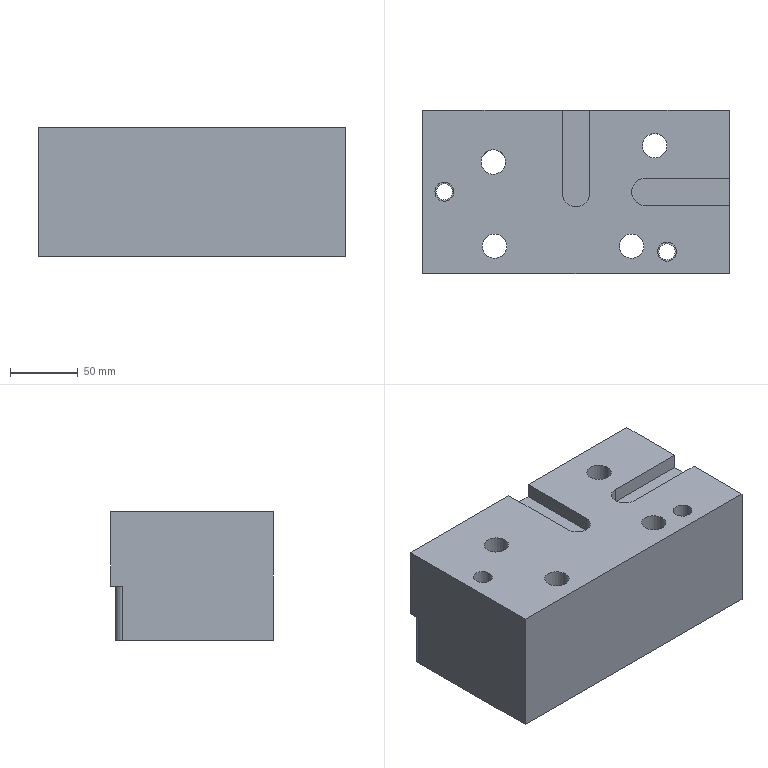Part | STEP file | lll_id3482_x_t | 1 solid | 113 faces | box 226 x 120 x 95 mm | volume 2052997 mm3 | plane 79 | cylinder 27 | cone 7 | commonest cylinder face diameters 10.506 x5 10 x4 18.009 x4 20 x4 26.007 x4 6.8 x2